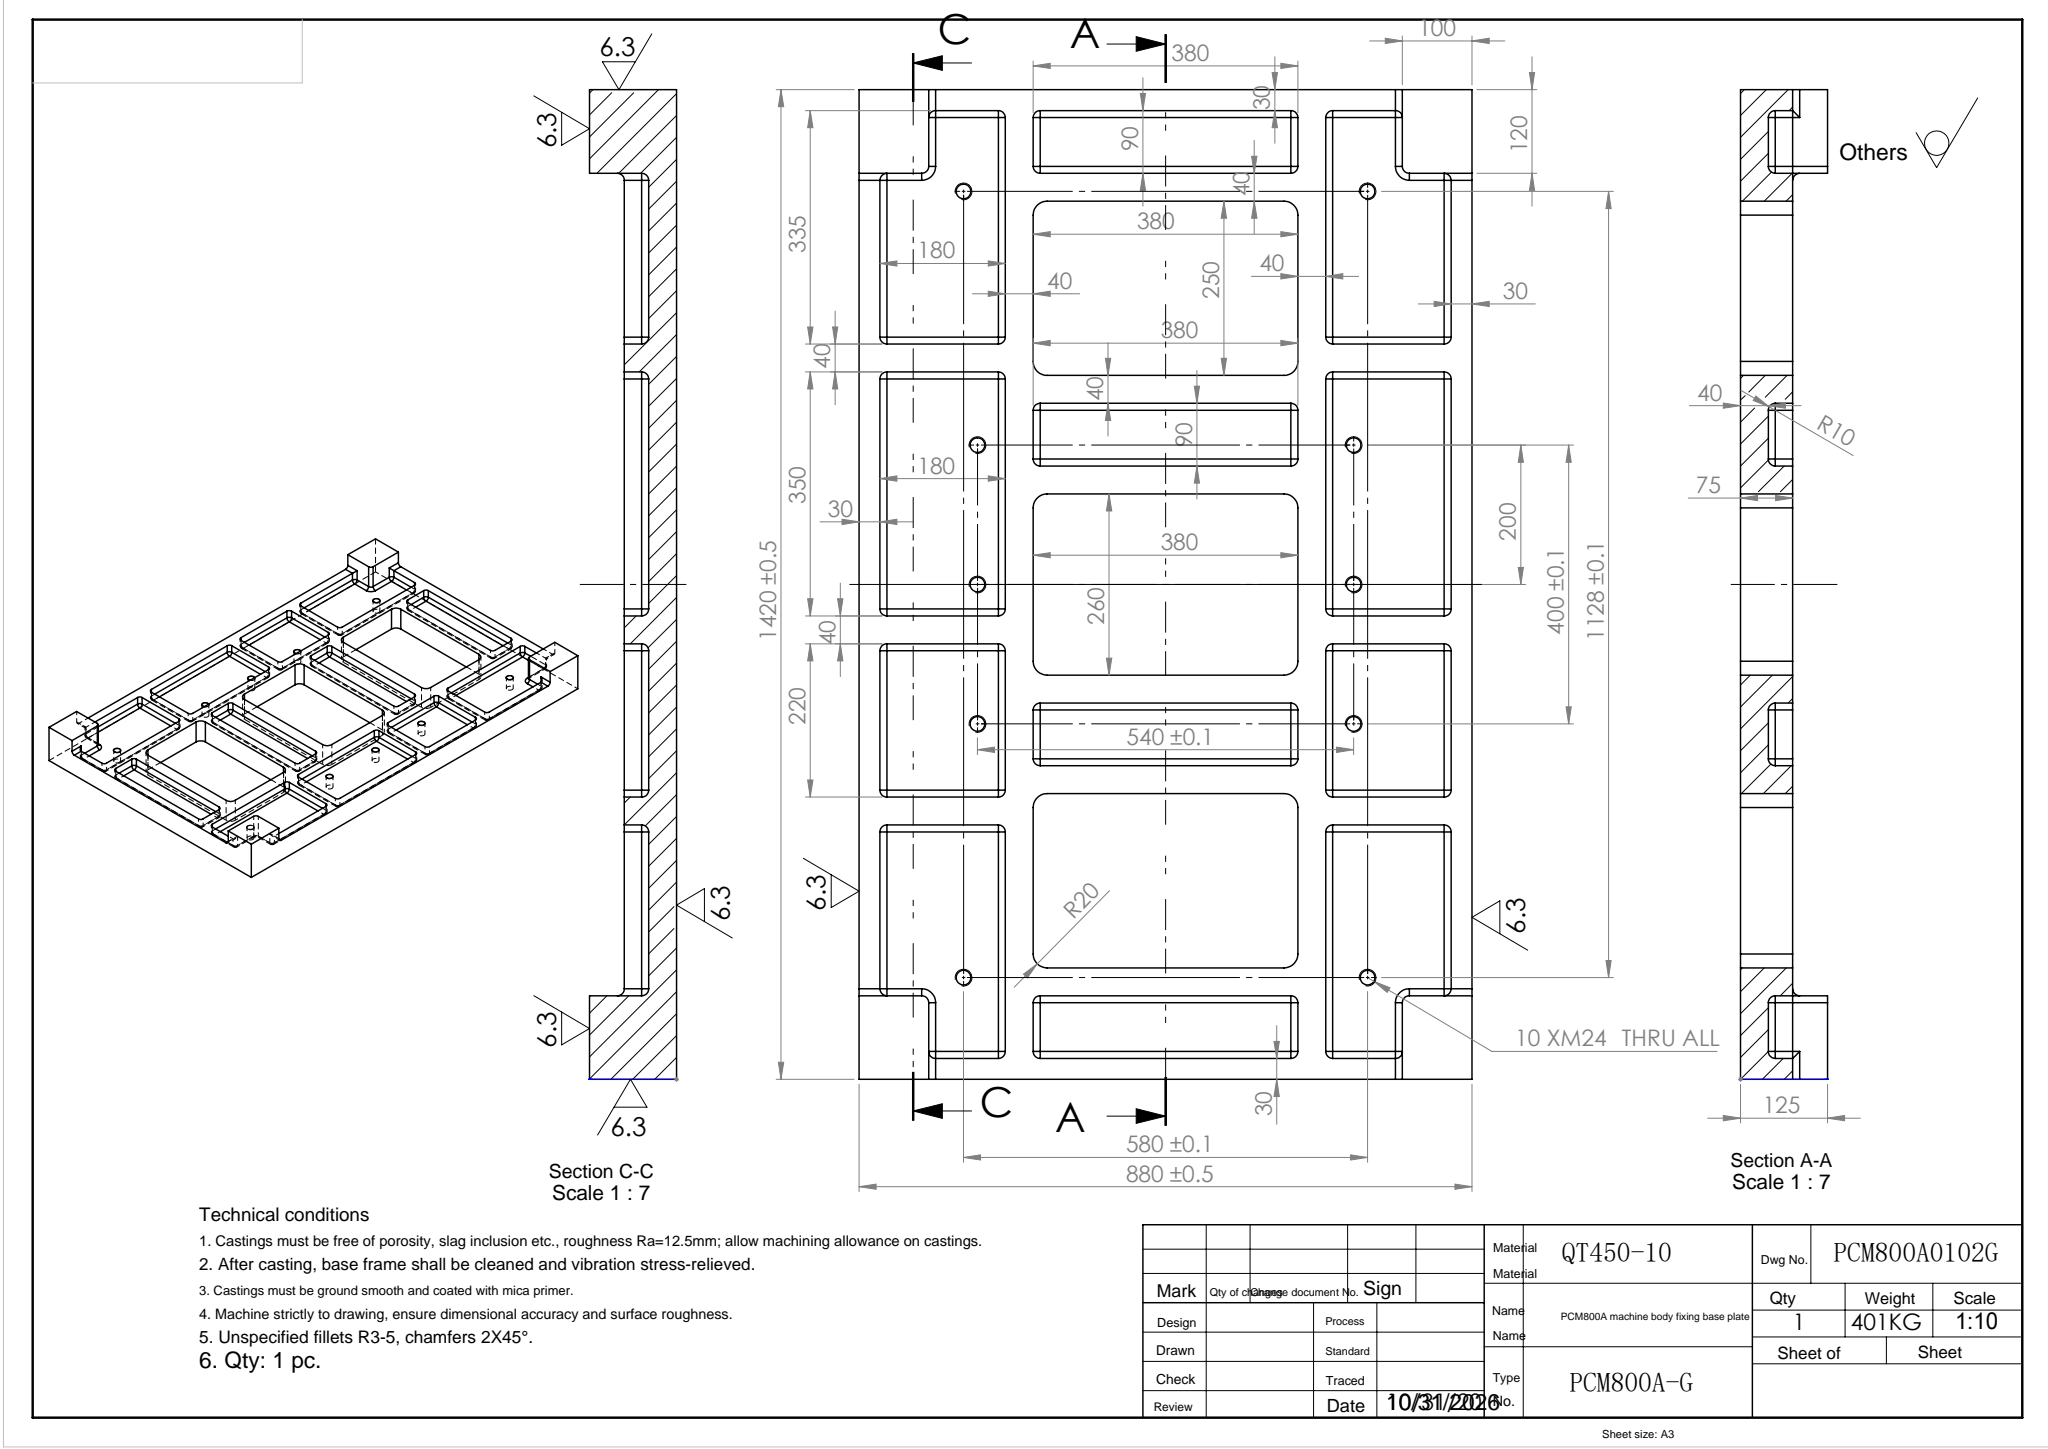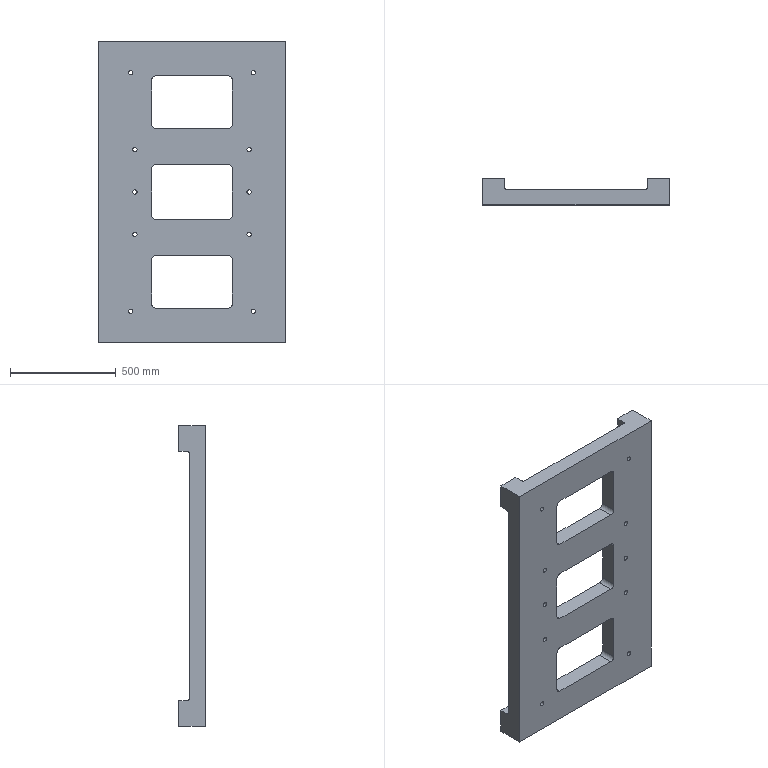Part | SolidWorks | features Fillet 3, 3DProfileFeature 2, Cut 2, HoleWzd 2, LPattern 2, Extrusion 1, ICE 1 | 1 solid | 298 faces | box 880 x 125 x 1420 mm | volume 55146557 mm3 | cylinder 152 | plane 90 | sphere 52 | torus 4 | commonest cylinder face diameters 20 x120 21 x20 40 x12